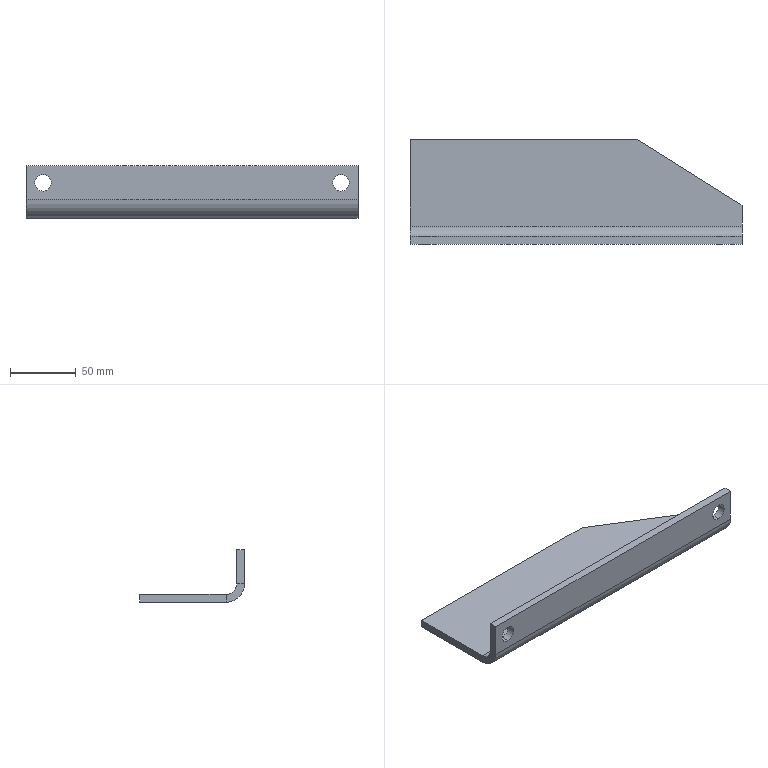Part | SolidWorks | features ICE 2, FlatPattern 1, SMBaseFlange 1, SheetMetal 1 | 1 solid | 19 faces | box 253 x 80 x 40 mm | volume 152413 mm3 | plane 13 | cylinder 6 | commonest cylinder face diameters 12.5 x4 16 x1 28 x1
STEP:
#1=CARTESIAN_POINT('',(240.,6.,20.75));
#2=VERTEX_POINT('',#1);
#3=CARTESIAN_POINT('',(240.,6.,33.25));
#4=VERTEX_POINT('',#3);
#5=CARTESIAN_POINT('',(240.,6.,27.));
#6=DIRECTION('',(0.,1.,0.));
#7=DIRECTION('',(0.,0.,-1.));
#8=AXIS2_PLACEMENT_3D('',#5,#6,#7);
#9=CIRCLE('',#8,6.25);
#10=EDGE_CURVE('',#2,#4,#9,.T.);
#11=ORIENTED_EDGE('',*,*,#10,.T.);
#12=CARTESIAN_POINT('',(240.,0.,33.25));
#13=VERTEX_POINT('',#12);
#14=CARTESIAN_POINT('',(240.,80.001,33.25));
#15=DIRECTION('',(0.,-1.,0.));
#16=VECTOR('',#15,1000.);
#17=LINE('',#14,#16);
#18=EDGE_CURVE('',#4,#13,#17,.T.);
#19=ORIENTED_EDGE('',*,*,#18,.T.);
#20=CARTESIAN_POINT('',(240.,0.,20.75));
#21=VERTEX_POINT('',#20);
#22=CARTESIAN_POINT('',(240.,0.,27.));
#23=DIRECTION('',(0.,-1.,0.));
#24=DIRECTION('',(0.,0.,-1.));
#25=AXIS2_PLACEMENT_3D('',#22,#23,#24);
#26=CIRCLE('',#25,6.25);
#27=EDGE_CURVE('',#13,#21,#26,.T.);
#28=ORIENTED_EDGE('',*,*,#27,.T.);
#29=CARTESIAN_POINT('',(240.,80.001,20.75));
#30=DIRECTION('',(0.,-1.,0.));
#31=VECTOR('',#30,1000.);
#32=LINE('',#29,#31);
#33=EDGE_CURVE('',#2,#21,#32,.T.);
#34=ORIENTED_EDGE('',*,*,#33,.F.);
#35=EDGE_LOOP('',(#11,#19,#28,#34));
#36=FACE_OUTER_BOUND('',#35,.T.);
#37=CARTESIAN_POINT('',(240.,80.001,27.));
#38=DIRECTION('',(0.,-1.,0.));
#39=DIRECTION('',(0.,0.,-1.));
#40=AXIS2_PLACEMENT_3D('',#37,#38,#39);
#41=CYLINDRICAL_SURFACE('',#40,6.25);
#42=ADVANCED_FACE('',(#36),#41,.F.);
#43=CARTESIAN_POINT('',(13.,6.,20.75));
#44=VERTEX_POINT('',#43);
#45=CARTESIAN_POINT('',(13.,6.,33.25));
#46=VERTEX_POINT('',#45);
#47=CARTESIAN_POINT('',(13.,6.,27.));
#48=DIRECTION('',(0.,1.,0.));
#49=DIRECTION('',(0.,0.,-1.));
#50=AXIS2_PLACEMENT_3D('',#47,#48,#49);
#51=CIRCLE('',#50,6.25);
#52=EDGE_CURVE('',#44,#46,#51,.T.);
#53=ORIENTED_EDGE('',*,*,#52,.T.);
#54=CARTESIAN_POINT('',(13.,0.,33.25));
#55=VERTEX_POINT('',#54);
#56=CARTESIAN_POINT('',(13.,80.001,33.25));
#57=DIRECTION('',(0.,-1.,0.));
#58=VECTOR('',#57,1000.);
#59=LINE('',#56,#58);
#60=EDGE_CURVE('',#46,#55,#59,.T.);
#61=ORIENTED_EDGE('',*,*,#60,.T.);
#62=CARTESIAN_POINT('',(13.,0.,20.75));
#63=VERTEX_POINT('',#62);
#64=CARTESIAN_POINT('',(13.,0.,27.));
#65=DIRECTION('',(0.,-1.,0.));
#66=DIRECTION('',(0.,0.,-1.));
#67=AXIS2_PLACEMENT_3D('',#64,#65,#66);
#68=CIRCLE('',#67,6.25);
#69=EDGE_CURVE('',#55,#63,#68,.T.);
#70=ORIENTED_EDGE('',*,*,#69,.T.);
#71=CARTESIAN_POINT('',(13.,80.001,20.75));
#72=DIRECTION('',(0.,-1.,0.));
#73=VECTOR('',#72,1000.);
#74=LINE('',#71,#73);
#75=EDGE_CURVE('',#44,#63,#74,.T.);
#76=ORIENTED_EDGE('',*,*,#75,.F.);
#77=EDGE_LOOP('',(#53,#61,#70,#76));
#78=FACE_OUTER_BOUND('',#77,.T.);
#79=CARTESIAN_POINT('',(13.,80.001,27.));
#80=DIRECTION('',(0.,-1.,0.));
#81=DIRECTION('',(0.,0.,-1.));
#82=AXIS2_PLACEMENT_3D('',#79,#80,#81);
#83=CYLINDRICAL_SURFACE('',#82,6.25);
#84=ADVANCED_FACE('',(#78),#83,.F.);
#85=CARTESIAN_POINT('',(173.,80.,0.));
#86=VERTEX_POINT('',#85);
#87=CARTESIAN_POINT('',(0.,80.,0.));
#88=VERTEX_POINT('',#87);
#89=CARTESIAN_POINT('',(253.,80.,0.));
#90=DIRECTION('',(-1.,0.,0.));
#91=VECTOR('',#90,1000.);
#92=LINE('',#89,#91);
#93=EDGE_CURVE('',#86,#88,#92,.T.);
#94=ORIENTED_EDGE('',*,*,#93,.F.);
#95=CARTESIAN_POINT('',(253.,30.,0.));
#96=VERTEX_POINT('',#95);
#97=CARTESIAN_POINT('',(173.,80.,0.));
#98=DIRECTION('',(0.848,-0.53,0.));
#99=VECTOR('',#98,1000.);
#100=LINE('',#97,#99);
#101=EDGE_CURVE('',#86,#96,#100,.T.);
#102=ORIENTED_EDGE('',*,*,#101,.T.);
#103=CARTESIAN_POINT('',(253.,14.,0.));
#104=VERTEX_POINT('',#103);
#105=CARTESIAN_POINT('',(253.,0.,0.));
#106=DIRECTION('',(0.,-1.,0.));
#107=VECTOR('',#106,1000.);
#108=LINE('',#105,#107);
#109=EDGE_CURVE('',#96,#104,#108,.T.);
#110=ORIENTED_EDGE('',*,*,#109,.T.);
#111=CARTESIAN_POINT('',(0.,14.,0.));
#112=VERTEX_POINT('',#111);
#113=CARTESIAN_POINT('',(253.,14.,0.));
#114=DIRECTION('',(-1.,0.,0.));
#115=VECTOR('',#114,1000.);
#116=LINE('',#113,#115);
#117=EDGE_CURVE('',#104,#112,#116,.T.);
#118=ORIENTED_EDGE('',*,*,#117,.T.);
#119=CARTESIAN_POINT('',(0.,0.,0.));
#120=DIRECTION('',(0.,-1.,0.));
#121=VECTOR('',#120,1000.);
#122=LINE('',#119,#121);
#123=EDGE_CURVE('',#88,#112,#122,.T.);
#124=ORIENTED_EDGE('',*,*,#123,.F.);
#125=EDGE_LOOP('',(#94,#102,#110,#118,#124));
#126=FACE_OUTER_BOUND('',#125,.T.);
#127=CARTESIAN_POINT('',(253.,0.,0.));
#128=DIRECTION('',(0.,0.,-1.));
#129=DIRECTION('',(-1.,0.,0.));
#130=AXIS2_PLACEMENT_3D('',#127,#128,#129);
#131=PLANE('',#130);
#132=ADVANCED_FACE('',(#126),#131,.T.);
#133=CARTESIAN_POINT('',(173.,80.,6.));
#134=VERTEX_POINT('',#133);
#135=CARTESIAN_POINT('',(0.,80.,6.));
#136=VERTEX_POINT('',#135);
#137=CARTESIAN_POINT('',(253.,80.,6.));
#138=DIRECTION('',(-1.,0.,0.));
#139=VECTOR('',#138,1000.);
#140=LINE('',#137,#139);
#141=EDGE_CURVE('',#134,#136,#140,.T.);
#142=ORIENTED_EDGE('',*,*,#141,.F.);
#143=CARTESIAN_POINT('',(173.,80.,0.));
#144=DIRECTION('',(0.,0.,1.));
#145=VECTOR('',#144,1000.);
#146=LINE('',#143,#145);
#147=EDGE_CURVE('',#86,#134,#146,.T.);
#148=ORIENTED_EDGE('',*,*,#147,.F.);
#149=ORIENTED_EDGE('',*,*,#93,.T.);
#150=CARTESIAN_POINT('',(0.,80.,6.));
#151=DIRECTION('',(0.,0.,-1.));
#152=VECTOR('',#151,1000.);
#153=LINE('',#150,#152);
#154=EDGE_CURVE('',#136,#88,#153,.T.);
#155=ORIENTED_EDGE('',*,*,#154,.F.);
#156=EDGE_LOOP('',(#142,#148,#149,#155));
#157=FACE_OUTER_BOUND('',#156,.T.);
#158=CARTESIAN_POINT('',(253.,80.,6.));
#159=DIRECTION('',(0.,1.,0.));
#160=DIRECTION('',(0.,0.,1.));
#161=AXIS2_PLACEMENT_3D('',#158,#159,#160);
#162=PLANE('',#161);
#163=ADVANCED_FACE('',(#157),#162,.T.);
#164=CARTESIAN_POINT('',(253.,30.,6.));
#165=VERTEX_POINT('',#164);
#166=CARTESIAN_POINT('',(173.,80.,6.));
#167=DIRECTION('',(0.848,-0.53,0.));
#168=VECTOR('',#167,1000.);
#169=LINE('',#166,#168);
#170=EDGE_CURVE('',#134,#165,#169,.T.);
#171=ORIENTED_EDGE('',*,*,#170,.F.);
#172=ORIENTED_EDGE('',*,*,#141,.T.);
#173=CARTESIAN_POINT('',(0.,14.,6.));
#174=VERTEX_POINT('',#173);
#175=CARTESIAN_POINT('',(0.,0.,6.));
#176=DIRECTION('',(0.,-1.,0.));
#177=VECTOR('',#176,1000.);
#178=LINE('',#175,#177);
#179=EDGE_CURVE('',#136,#174,#178,.T.);
#180=ORIENTED_EDGE('',*,*,#179,.T.);
#181=CARTESIAN_POINT('',(253.,14.,6.));
#182=VERTEX_POINT('',#181);
#183=CARTESIAN_POINT('',(253.,14.,6.));
#184=DIRECTION('',(-1.,0.,0.));
#185=VECTOR('',#184,1000.);
#186=LINE('',#183,#185);
#187=EDGE_CURVE('',#182,#174,#186,.T.);
#188=ORIENTED_EDGE('',*,*,#187,.F.);
#189=CARTESIAN_POINT('',(253.,0.,6.));
#190=DIRECTION('',(0.,-1.,0.));
#191=VECTOR('',#190,1000.);
#192=LINE('',#189,#191);
#193=EDGE_CURVE('',#165,#182,#192,.T.);
#194=ORIENTED_EDGE('',*,*,#193,.F.);
#195=EDGE_LOOP('',(#171,#172,#180,#188,#194));
#196=FACE_OUTER_BOUND('',#195,.T.);
#197=CARTESIAN_POINT('',(253.,0.,6.));
#198=DIRECTION('',(0.,0.,-1.));
#199=DIRECTION('',(-1.,0.,0.));
#200=AXIS2_PLACEMENT_3D('',#197,#198,#199);
#201=PLANE('',#200);
#202=ADVANCED_FACE('',(#196),#201,.F.);
#203=ORIENTED_EDGE('',*,*,#109,.F.);
#204=CARTESIAN_POINT('',(253.,30.,0.));
#205=DIRECTION('',(0.,0.,1.));
#206=VECTOR('',#205,1000.);
#207=LINE('',#204,#206);
#208=EDGE_CURVE('',#96,#165,#207,.T.);
#209=ORIENTED_EDGE('',*,*,#208,.T.);
#210=ORIENTED_EDGE('',*,*,#193,.T.);
#211=CARTESIAN_POINT('',(253.,14.,6.));
#212=DIRECTION('',(0.,0.,-1.));
#213=VECTOR('',#212,1000.);
#214=LINE('',#211,#213);
#215=EDGE_CURVE('',#182,#104,#214,.T.);
#216=ORIENTED_EDGE('',*,*,#215,.T.);
#217=EDGE_LOOP('',(#203,#209,#210,#216));
#218=FACE_OUTER_BOUND('',#217,.T.);
#219=CARTESIAN_POINT('',(253.,14.,14.));
#220=DIRECTION('',(1.,0.,0.));
#221=DIRECTION('',(0.,0.,-1.));
#222=AXIS2_PLACEMENT_3D('',#219,#220,#221);
#223=PLANE('',#222);
#224=ADVANCED_FACE('',(#218),#223,.T.);
#225=CARTESIAN_POINT('',(253.,0.,14.));
#226=VERTEX_POINT('',#225);
#227=CARTESIAN_POINT('',(253.,6.,14.));
#228=VERTEX_POINT('',#227);
#229=CARTESIAN_POINT('',(253.,0.,14.));
#230=DIRECTION('',(0.,1.,0.));
#231=VECTOR('',#230,1000.);
#232=LINE('',#229,#231);
#233=EDGE_CURVE('',#226,#228,#232,.T.);
#234=ORIENTED_EDGE('',*,*,#233,.F.);
#235=CARTESIAN_POINT('',(253.,14.,14.));
#236=DIRECTION('',(-1.,0.,0.));
#237=DIRECTION('',(0.,0.,-1.));
#238=AXIS2_PLACEMENT_3D('',#235,#236,#237);
#239=CIRCLE('',#238,14.);
#240=EDGE_CURVE('',#104,#226,#239,.T.);
#241=ORIENTED_EDGE('',*,*,#240,.F.);
#242=ORIENTED_EDGE('',*,*,#215,.F.);
#243=CARTESIAN_POINT('',(253.,14.,14.));
#244=DIRECTION('',(-1.,0.,0.));
#245=DIRECTION('',(0.,0.,-1.));
#246=AXIS2_PLACEMENT_3D('',#243,#244,#245);
#247=CIRCLE('',#246,8.);
#248=EDGE_CURVE('',#182,#228,#247,.T.);
#249=ORIENTED_EDGE('',*,*,#248,.T.);
#250=EDGE_LOOP('',(#234,#241,#242,#249));
#251=FACE_OUTER_BOUND('',#250,.T.);
#252=CARTESIAN_POINT('',(253.,0.,14.));
#253=DIRECTION('',(1.,0.,0.));
#254=DIRECTION('',(0.,0.,-1.));
#255=AXIS2_PLACEMENT_3D('',#252,#253,#254);
#256=PLANE('',#255);
#257=ADVANCED_FACE('',(#251),#256,.T.);
#258=CARTESIAN_POINT('',(253.,0.,40.));
#259=VERTEX_POINT('',#258);
#260=CARTESIAN_POINT('',(253.,0.,0.));
#261=DIRECTION('',(0.,0.,1.));
#262=VECTOR('',#261,1000.);
#263=LINE('',#260,#262);
#264=EDGE_CURVE('',#226,#259,#263,.T.);
#265=ORIENTED_EDGE('',*,*,#264,.F.);
#266=ORIENTED_EDGE('',*,*,#233,.T.);
#267=CARTESIAN_POINT('',(253.,6.,40.));
#268=VERTEX_POINT('',#267);
#269=CARTESIAN_POINT('',(253.,6.,0.));
#270=DIRECTION('',(0.,0.,1.));
#271=VECTOR('',#270,1000.);
#272=LINE('',#269,#271);
#273=EDGE_CURVE('',#228,#268,#272,.T.);
#274=ORIENTED_EDGE('',*,*,#273,.T.);
#275=CARTESIAN_POINT('',(253.,0.,40.));
#276=DIRECTION('',(0.,1.,0.));
#277=VECTOR('',#276,1000.);
#278=LINE('',#275,#277);
#279=EDGE_CURVE('',#259,#268,#278,.T.);
#280=ORIENTED_EDGE('',*,*,#279,.F.);
#281=EDGE_LOOP('',(#265,#266,#274,#280));
#282=FACE_OUTER_BOUND('',#281,.T.);
#283=CARTESIAN_POINT('',(253.,14.,6.));
#284=DIRECTION('',(1.,0.,0.));
#285=DIRECTION('',(0.,0.,-1.));
#286=AXIS2_PLACEMENT_3D('',#283,#284,#285);
#287=PLANE('',#286);
#288=ADVANCED_FACE('',(#282),#287,.T.);
#289=CARTESIAN_POINT('',(0.,14.,0.));
#290=DIRECTION('',(0.,0.,1.));
#291=VECTOR('',#290,1000.);
#292=LINE('',#289,#291);
#293=EDGE_CURVE('',#112,#174,#292,.T.);
#294=ORIENTED_EDGE('',*,*,#293,.F.);
#295=CARTESIAN_POINT('',(0.,0.,14.));
#296=VERTEX_POINT('',#295);
#297=CARTESIAN_POINT('',(0.,14.,14.));
#298=DIRECTION('',(-1.,0.,0.));
#299=DIRECTION('',(0.,0.,-1.));
#300=AXIS2_PLACEMENT_3D('',#297,#298,#299);
#301=CIRCLE('',#300,14.);
#302=EDGE_CURVE('',#112,#296,#301,.T.);
#303=ORIENTED_EDGE('',*,*,#302,.T.);
#304=CARTESIAN_POINT('',(0.,6.,14.));
#305=VERTEX_POINT('',#304);
#306=CARTESIAN_POINT('',(0.,6.,14.));
#307=DIRECTION('',(0.,-1.,0.));
#308=VECTOR('',#307,1000.);
#309=LINE('',#306,#308);
#310=EDGE_CURVE('',#305,#296,#309,.T.);
#311=ORIENTED_EDGE('',*,*,#310,.F.);
#312=CARTESIAN_POINT('',(0.,14.,14.));
#313=DIRECTION('',(-1.,0.,0.));
#314=DIRECTION('',(0.,0.,-1.));
#315=AXIS2_PLACEMENT_3D('',#312,#313,#314);
#316=CIRCLE('',#315,8.);
#317=EDGE_CURVE('',#174,#305,#316,.T.);
#318=ORIENTED_EDGE('',*,*,#317,.F.);
#319=EDGE_LOOP('',(#294,#303,#311,#318));
#320=FACE_OUTER_BOUND('',#319,.T.);
#321=CARTESIAN_POINT('',(0.,14.,0.));
#322=DIRECTION('',(-1.,0.,0.));
#323=DIRECTION('',(0.,0.,1.));
#324=AXIS2_PLACEMENT_3D('',#321,#322,#323);
#325=PLANE('',#324);
#326=ADVANCED_FACE('',(#320),#325,.T.);
#327=ORIENTED_EDGE('',*,*,#123,.T.);
#328=ORIENTED_EDGE('',*,*,#293,.T.);
#329=ORIENTED_EDGE('',*,*,#179,.F.);
#330=ORIENTED_EDGE('',*,*,#154,.T.);
#331=EDGE_LOOP('',(#327,#328,#329,#330));
#332=FACE_OUTER_BOUND('',#331,.T.);
#333=CARTESIAN_POINT('',(0.,6.,14.));
#334=DIRECTION('',(-1.,0.,0.));
#335=DIRECTION('',(0.,0.,1.));
#336=AXIS2_PLACEMENT_3D('',#333,#334,#335);
#337=PLANE('',#336);
#338=ADVANCED_FACE('',(#332),#337,.T.);
#339=ORIENTED_EDGE('',*,*,#10,.F.);
#340=CARTESIAN_POINT('',(240.,6.,27.));
#341=DIRECTION('',(0.,1.,0.));
#342=DIRECTION('',(0.,0.,-1.));
#343=AXIS2_PLACEMENT_3D('',#340,#341,#342);
#344=CIRCLE('',#343,6.25);
#345=EDGE_CURVE('',#4,#2,#344,.T.);
#346=ORIENTED_EDGE('',*,*,#345,.F.);
#347=EDGE_LOOP('',(#339,#346));
#348=FACE_BOUND('',#347,.T.);
#349=ORIENTED_EDGE('',*,*,#52,.F.);
#350=CARTESIAN_POINT('',(13.,6.,27.));
#351=DIRECTION('',(0.,1.,0.));
#352=DIRECTION('',(0.,0.,-1.));
#353=AXIS2_PLACEMENT_3D('',#350,#351,#352);
#354=CIRCLE('',#353,6.25);
#355=EDGE_CURVE('',#46,#44,#354,.T.);
#356=ORIENTED_EDGE('',*,*,#355,.F.);
#357=EDGE_LOOP('',(#349,#356));
#358=FACE_BOUND('',#357,.T.);
#359=CARTESIAN_POINT('',(0.,6.,40.));
#360=VERTEX_POINT('',#359);
#361=CARTESIAN_POINT('',(0.,6.,0.));
#362=DIRECTION('',(0.,0.,1.));
#363=VECTOR('',#362,1000.);
#364=LINE('',#361,#363);
#365=EDGE_CURVE('',#305,#360,#364,.T.);
#366=ORIENTED_EDGE('',*,*,#365,.T.);
#367=CARTESIAN_POINT('',(253.,6.,40.));
#368=DIRECTION('',(-1.,0.,0.));
#369=VECTOR('',#368,1000.);
#370=LINE('',#367,#369);
#371=EDGE_CURVE('',#268,#360,#370,.T.);
#372=ORIENTED_EDGE('',*,*,#371,.F.);
#373=ORIENTED_EDGE('',*,*,#273,.F.);
#374=CARTESIAN_POINT('',(253.,6.,14.));
#375=DIRECTION('',(-1.,0.,0.));
#376=VECTOR('',#375,1000.);
#377=LINE('',#374,#376);
#378=EDGE_CURVE('',#228,#305,#377,.T.);
#379=ORIENTED_EDGE('',*,*,#378,.T.);
#380=EDGE_LOOP('',(#366,#372,#373,#379));
#381=FACE_OUTER_BOUND('',#380,.T.);
#382=CARTESIAN_POINT('',(253.,6.,0.));
#383=DIRECTION('',(0.,-1.,0.));
#384=DIRECTION('',(0.,0.,-1.));
#385=AXIS2_PLACEMENT_3D('',#382,#383,#384);
#386=PLANE('',#385);
#387=ADVANCED_FACE('',(#348,#358,#381),#386,.F.);
#388=CARTESIAN_POINT('',(0.,0.,40.));
#389=VERTEX_POINT('',#388);
#390=CARTESIAN_POINT('',(0.,0.,40.));
#391=DIRECTION('',(0.,1.,0.));
#392=VECTOR('',#391,1000.);
#393=LINE('',#390,#392);
#394=EDGE_CURVE('',#389,#360,#393,.T.);
#395=ORIENTED_EDGE('',*,*,#394,.F.);
#396=CARTESIAN_POINT('',(253.,0.,40.));
#397=DIRECTION('',(-1.,0.,0.));
#398=VECTOR('',#397,1000.);
#399=LINE('',#396,#398);
#400=EDGE_CURVE('',#259,#389,#399,.T.);
#401=ORIENTED_EDGE('',*,*,#400,.F.);
#402=ORIENTED_EDGE('',*,*,#279,.T.);
#403=ORIENTED_EDGE('',*,*,#371,.T.);
#404=EDGE_LOOP('',(#395,#401,#402,#403));
#405=FACE_OUTER_BOUND('',#404,.T.);
#406=CARTESIAN_POINT('',(253.,0.,40.));
#407=DIRECTION('',(0.,0.,1.));
#408=DIRECTION('',(1.,0.,0.));
#409=AXIS2_PLACEMENT_3D('',#406,#407,#408);
#410=PLANE('',#409);
#411=ADVANCED_FACE('',(#405),#410,.T.);
#412=CARTESIAN_POINT('',(240.,0.,27.));
#413=DIRECTION('',(0.,-1.,0.));
#414=DIRECTION('',(0.,0.,-1.));
#415=AXIS2_PLACEMENT_3D('',#412,#413,#414);
#416=CIRCLE('',#415,6.25);
#417=EDGE_CURVE('',#21,#13,#416,.T.);
#418=ORIENTED_EDGE('',*,*,#417,.F.);
#419=ORIENTED_EDGE('',*,*,#27,.F.);
#420=EDGE_LOOP('',(#418,#419));
#421=FACE_BOUND('',#420,.T.);
#422=CARTESIAN_POINT('',(13.,0.,27.));
#423=DIRECTION('',(0.,-1.,0.));
#424=DIRECTION('',(0.,0.,-1.));
#425=AXIS2_PLACEMENT_3D('',#422,#423,#424);
#426=CIRCLE('',#425,6.25);
#427=EDGE_CURVE('',#63,#55,#426,.T.);
#428=ORIENTED_EDGE('',*,*,#427,.F.);
#429=ORIENTED_EDGE('',*,*,#69,.F.);
#430=EDGE_LOOP('',(#428,#429));
#431=FACE_BOUND('',#430,.T.);
#432=CARTESIAN_POINT('',(0.,0.,0.));
#433=DIRECTION('',(0.,0.,1.));
#434=VECTOR('',#433,1000.);
#435=LINE('',#432,#434);
#436=EDGE_CURVE('',#296,#389,#435,.T.);
#437=ORIENTED_EDGE('',*,*,#436,.F.);
#438=CARTESIAN_POINT('',(253.,0.,14.));
#439=DIRECTION('',(-1.,0.,0.));
#440=VECTOR('',#439,1000.);
#441=LINE('',#438,#440);
#442=EDGE_CURVE('',#226,#296,#441,.T.);
#443=ORIENTED_EDGE('',*,*,#442,.F.);
#444=ORIENTED_EDGE('',*,*,#264,.T.);
#445=ORIENTED_EDGE('',*,*,#400,.T.);
#446=EDGE_LOOP('',(#437,#443,#444,#445));
#447=FACE_OUTER_BOUND('',#446,.T.);
#448=CARTESIAN_POINT('',(253.,0.,0.));
#449=DIRECTION('',(0.,-1.,0.));
#450=DIRECTION('',(0.,0.,-1.));
#451=AXIS2_PLACEMENT_3D('',#448,#449,#450);
#452=PLANE('',#451);
#453=ADVANCED_FACE('',(#421,#431,#447),#452,.T.);
#454=ORIENTED_EDGE('',*,*,#302,.F.);
#455=ORIENTED_EDGE('',*,*,#117,.F.);
#456=ORIENTED_EDGE('',*,*,#240,.T.);
#457=ORIENTED_EDGE('',*,*,#442,.T.);
#458=EDGE_LOOP('',(#454,#455,#456,#457));
#459=FACE_OUTER_BOUND('',#458,.T.);
#460=CARTESIAN_POINT('',(253.,14.,14.));
#461=DIRECTION('',(-1.,0.,0.));
#462=DIRECTION('',(0.,0.,1.));
#463=AXIS2_PLACEMENT_3D('',#460,#461,#462);
#464=CYLINDRICAL_SURFACE('',#463,14.);
#465=ADVANCED_FACE('',(#459),#464,.T.);
#466=ORIENTED_EDGE('',*,*,#317,.T.);
#467=ORIENTED_EDGE('',*,*,#378,.F.);
#468=ORIENTED_EDGE('',*,*,#248,.F.);
#469=ORIENTED_EDGE('',*,*,#187,.T.);
#470=EDGE_LOOP('',(#466,#467,#468,#469));
#471=FACE_OUTER_BOUND('',#470,.T.);
#472=CARTESIAN_POINT('',(253.,14.,14.));
#473=DIRECTION('',(-1.,0.,0.));
#474=DIRECTION('',(0.,0.,1.));
#475=AXIS2_PLACEMENT_3D('',#472,#473,#474);
#476=CYLINDRICAL_SURFACE('',#475,8.);
#477=ADVANCED_FACE('',(#471),#476,.F.);
#478=ORIENTED_EDGE('',*,*,#365,.F.);
#479=ORIENTED_EDGE('',*,*,#310,.T.);
#480=ORIENTED_EDGE('',*,*,#436,.T.);
#481=ORIENTED_EDGE('',*,*,#394,.T.);
#482=EDGE_LOOP('',(#478,#479,#480,#481));
#483=FACE_OUTER_BOUND('',#482,.T.);
#484=CARTESIAN_POINT('',(0.,14.,14.));
#485=DIRECTION('',(1.,0.,0.));
#486=DIRECTION('',(0.,0.,-1.));
#487=AXIS2_PLACEMENT_3D('',#484,#485,#486);
#488=PLANE('',#487);
#489=ADVANCED_FACE('',(#483),#488,.F.);
#490=ORIENTED_EDGE('',*,*,#60,.F.);
#491=ORIENTED_EDGE('',*,*,#355,.T.);
#492=ORIENTED_EDGE('',*,*,#75,.T.);
#493=ORIENTED_EDGE('',*,*,#427,.T.);
#494=EDGE_LOOP('',(#490,#491,#492,#493));
#495=FACE_OUTER_BOUND('',#494,.T.);
#496=CARTESIAN_POINT('',(13.,80.001,27.));
#497=DIRECTION('',(0.,-1.,0.));
#498=DIRECTION('',(0.,0.,-1.));
#499=AXIS2_PLACEMENT_3D('',#496,#497,#498);
#500=CYLINDRICAL_SURFACE('',#499,6.25);
#501=ADVANCED_FACE('',(#495),#500,.F.);
#502=ORIENTED_EDGE('',*,*,#18,.F.);
#503=ORIENTED_EDGE('',*,*,#345,.T.);
#504=ORIENTED_EDGE('',*,*,#33,.T.);
#505=ORIENTED_EDGE('',*,*,#417,.T.);
#506=EDGE_LOOP('',(#502,#503,#504,#505));
#507=FACE_OUTER_BOUND('',#506,.T.);
#508=CARTESIAN_POINT('',(240.,80.001,27.));
#509=DIRECTION('',(0.,-1.,0.));
#510=DIRECTION('',(0.,0.,-1.));
#511=AXIS2_PLACEMENT_3D('',#508,#509,#510);
#512=CYLINDRICAL_SURFACE('',#511,6.25);
#513=ADVANCED_FACE('',(#507),#512,.F.);
#514=ORIENTED_EDGE('',*,*,#101,.F.);
#515=ORIENTED_EDGE('',*,*,#147,.T.);
#516=ORIENTED_EDGE('',*,*,#170,.T.);
#517=ORIENTED_EDGE('',*,*,#208,.F.);
#518=EDGE_LOOP('',(#514,#515,#516,#517));
#519=FACE_OUTER_BOUND('',#518,.T.);
#520=CARTESIAN_POINT('',(173.,80.,0.));
#521=DIRECTION('',(0.53,0.848,0.));
#522=DIRECTION('',(0.848,-0.53,0.));
#523=AXIS2_PLACEMENT_3D('',#520,#521,#522);
#524=PLANE('',#523);
#525=ADVANCED_FACE('',(#519),#524,.T.);
#526=CLOSED_SHELL('',(#42,#84,#132,#163,#202,#224,#257,#288,#326,#338,#387,#411,#453,#465,#477,#489,#501,#513,#525));
#527=MANIFOLD_SOLID_BREP('',#526);
#528=CARTESIAN_POINT('',(0.,0.,0.));
#529=DIRECTION('',(0.,0.,1.));
#530=DIRECTION('',(1.,0.,0.));
#531=AXIS2_PLACEMENT_3D('',#528,#529,#530);
#532=(LENGTH_UNIT()NAMED_UNIT(*)SI_UNIT(.MILLI.,.METRE.));
#533=UNCERTAINTY_MEASURE_WITH_UNIT(LENGTH_MEASURE(0.00001),#532,'','');
#534=(NAMED_UNIT(*)PLANE_ANGLE_UNIT()SI_UNIT($,.RADIAN.));
#535=(NAMED_UNIT(*)SI_UNIT($,.STERADIAN.)SOLID_ANGLE_UNIT());
#536=(GEOMETRIC_REPRESENTATION_CONTEXT(3)GLOBAL_UNCERTAINTY_ASSIGNED_CONTEXT((#533))GLOBAL_UNIT_ASSIGNED_CONTEXT((#532,#534,#535))REPRESENTATION_CONTEXT('',''));
#537=ADVANCED_BREP_SHAPE_REPRESENTATION('',(#527,#531),#536);